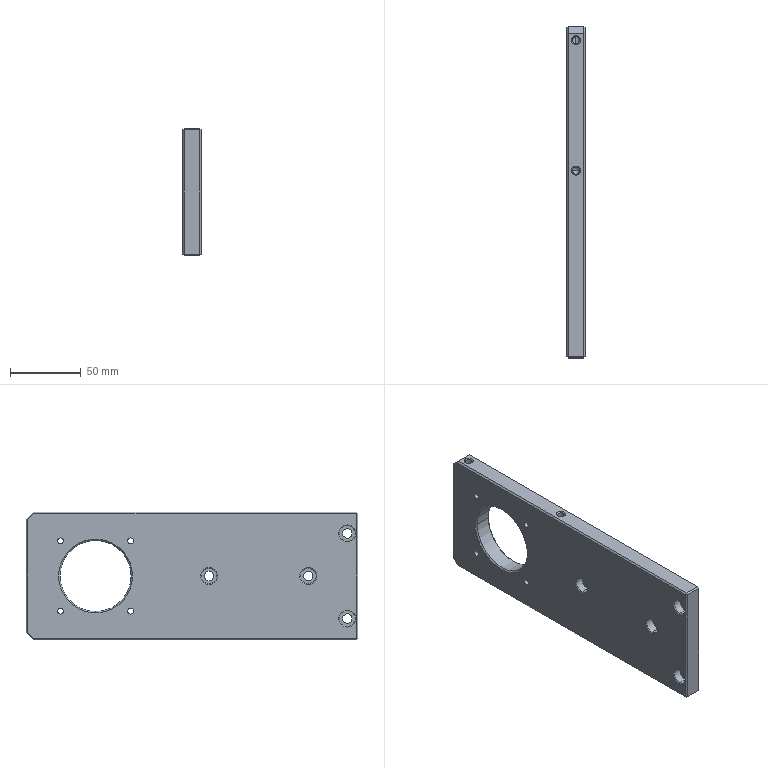Part | SolidWorks | features HoleWzd 5, Chamfer 3, ICE 2, Extrusion 1, Fillet 1, MirrorPattern 1, MoveFace 1 | 1 solid | 114 faces | box 13 x 234 x 90 mm | volume 241107 mm3 | cone 46 | cylinder 38 | plane 30 | commonest cylinder face diameters 5 x12 4.2 x8 6.6 x8 11 x8 50.1 x2